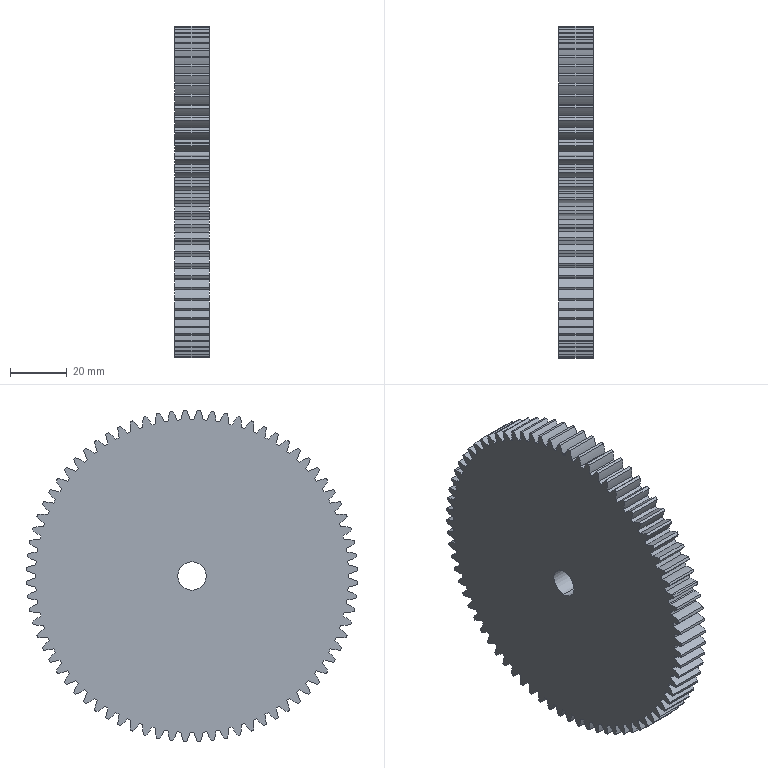Part | SolidWorks | features Boss 3, Cut 3, CirPattern 2, Fillet 2, Revolution 1 | 1 solid | 313 faces | box 12 x 116.937 x 116.937 mm | volume 120543 mm3 | cylinder 311 | plane 2 | commonest cylinder face diameters 45.6 x156 110.248 x77 117 x76 10 x2